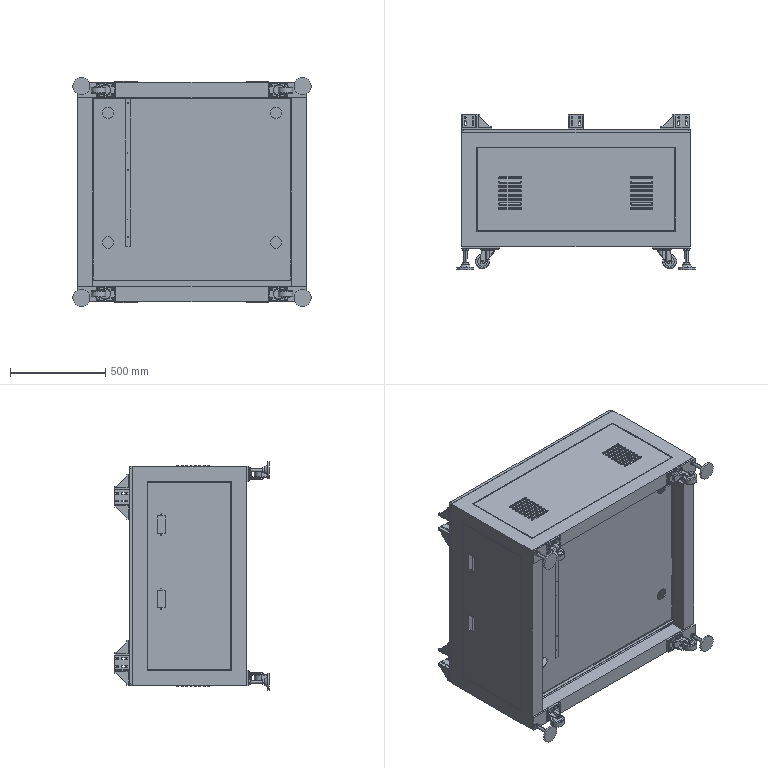Part | NX | 40 solids | 3394 faces | volume 96365724 mm3 | plane 1815 | cylinder 1113 | cone 210 | sphere 140 | spline 64 | torus 52 | commonest cylinder face diameters 9 x256 10 x192 12 x112 4 x98 2 x78 3.3 x54